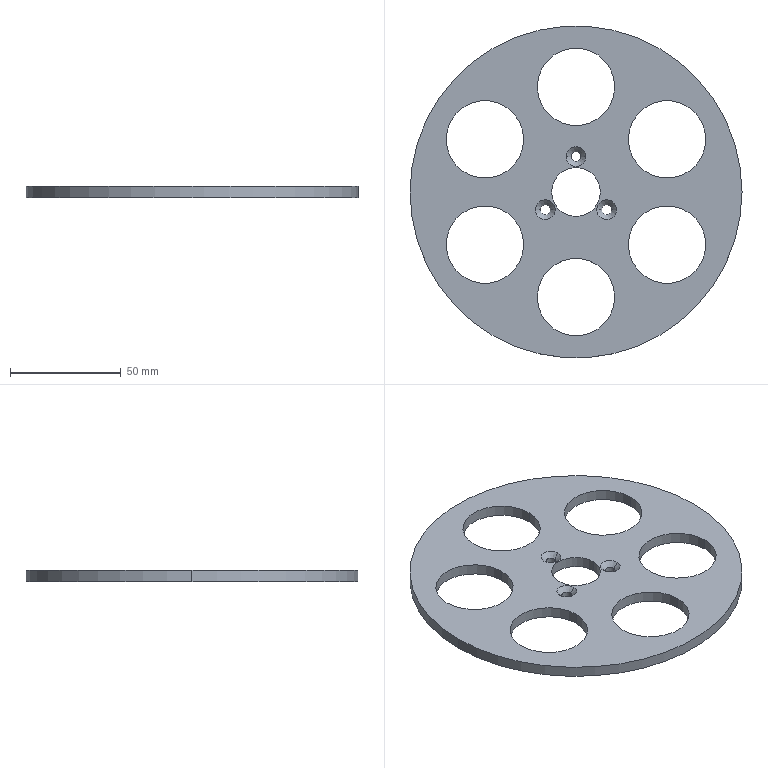Part | STEP file | QA-FC12 | 1 solid | 30 faces | box 150 x 150 x 5 mm | volume 57214 mm3 | cylinder 22 | cone 6 | plane 2 | commonest cylinder face diameters 35 x12 4.5 x6 22 x2 150 x2